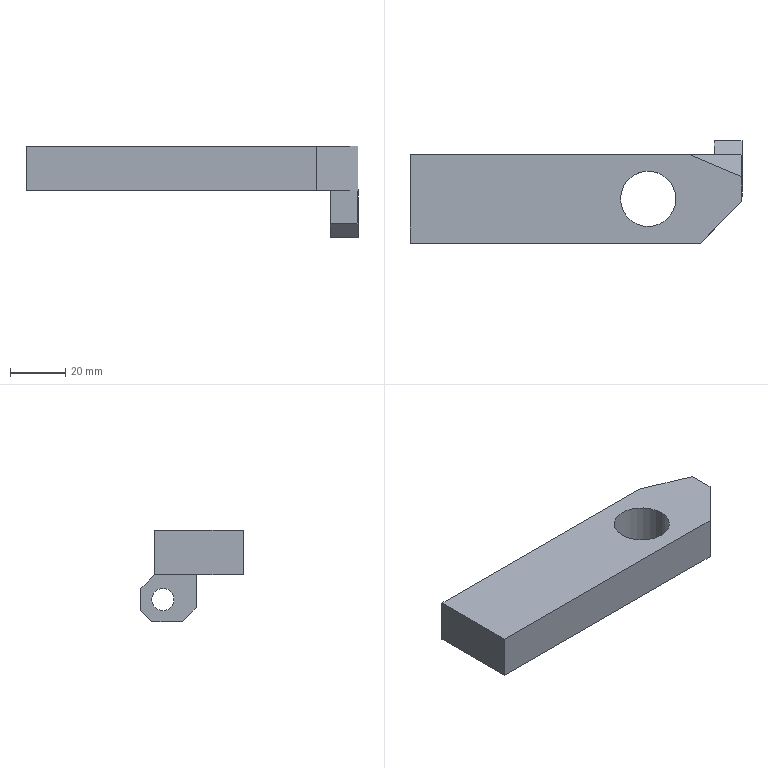Part | STEP file | [Anti-tilt]-Part-4 | 1 solid | 19 faces | box 120 x 37 x 33 mm | volume 56775 mm3 | plane 15 | cylinder 4 | commonest cylinder face diameters 8 x2 20 x2
STEP:
#1=CARTESIAN_POINT('',(63.91,-10.5,7.));
#2=VERTEX_POINT('',#1);
#3=CARTESIAN_POINT('',(63.91,-10.5,15.));
#4=VERTEX_POINT('',#3);
#5=CARTESIAN_POINT('',(63.91,-10.5,11.));
#6=DIRECTION('',(-1.,0.,0.));
#7=DIRECTION('',(0.,-1.,0.));
#8=AXIS2_PLACEMENT_3D('',#5,#6,#7);
#9=CIRCLE('',#8,4.);
#10=EDGE_CURVE('',#2,#4,#9,.T.);
#11=ORIENTED_EDGE('',*,*,#10,.F.);
#12=CARTESIAN_POINT('',(53.91,-10.5,7.));
#13=VERTEX_POINT('',#12);
#14=CARTESIAN_POINT('',(44.003,-10.5,7.));
#15=DIRECTION('',(-1.,0.,0.));
#16=VECTOR('',#15,1000.);
#17=LINE('',#14,#16);
#18=EDGE_CURVE('',#2,#13,#17,.T.);
#19=ORIENTED_EDGE('',*,*,#18,.T.);
#20=CARTESIAN_POINT('',(53.91,-10.5,15.));
#21=VERTEX_POINT('',#20);
#22=CARTESIAN_POINT('',(53.91,-10.5,11.));
#23=DIRECTION('',(1.,0.,0.));
#24=DIRECTION('',(0.,1.,0.));
#25=AXIS2_PLACEMENT_3D('',#22,#23,#24);
#26=CIRCLE('',#25,4.);
#27=EDGE_CURVE('',#21,#13,#26,.T.);
#28=ORIENTED_EDGE('',*,*,#27,.F.);
#29=CARTESIAN_POINT('',(44.003,-10.5,15.));
#30=DIRECTION('',(-1.,0.,0.));
#31=VECTOR('',#30,1000.);
#32=LINE('',#29,#31);
#33=EDGE_CURVE('',#4,#21,#32,.T.);
#34=ORIENTED_EDGE('',*,*,#33,.F.);
#35=EDGE_LOOP('',(#11,#19,#28,#34));
#36=FACE_OUTER_BOUND('',#35,.T.);
#37=CARTESIAN_POINT('',(44.003,-10.5,11.));
#38=DIRECTION('',(-1.,0.,0.));
#39=DIRECTION('',(0.,0.,1.));
#40=AXIS2_PLACEMENT_3D('',#37,#38,#39);
#41=CYLINDRICAL_SURFACE('',#40,4.);
#42=ADVANCED_FACE('',(#36),#41,.F.);
#43=CARTESIAN_POINT('',(40.003,-23.5,20.));
#44=VERTEX_POINT('',#43);
#45=CARTESIAN_POINT('',(20.003,-23.5,20.));
#46=VERTEX_POINT('',#45);
#47=CARTESIAN_POINT('',(30.003,-23.5,20.));
#48=DIRECTION('',(0.,0.,1.));
#49=DIRECTION('',(-1.,0.,0.));
#50=AXIS2_PLACEMENT_3D('',#47,#48,#49);
#51=CIRCLE('',#50,10.);
#52=EDGE_CURVE('',#44,#46,#51,.T.);
#53=ORIENTED_EDGE('',*,*,#52,.F.);
#54=CARTESIAN_POINT('',(40.003,-23.5,36.));
#55=VERTEX_POINT('',#54);
#56=CARTESIAN_POINT('',(40.003,-23.5,20.));
#57=DIRECTION('',(0.,0.,1.));
#58=VECTOR('',#57,1000.);
#59=LINE('',#56,#58);
#60=EDGE_CURVE('',#44,#55,#59,.T.);
#61=ORIENTED_EDGE('',*,*,#60,.T.);
#62=CARTESIAN_POINT('',(20.003,-23.5,36.));
#63=VERTEX_POINT('',#62);
#64=CARTESIAN_POINT('',(30.003,-23.5,36.));
#65=DIRECTION('',(0.,0.,1.));
#66=DIRECTION('',(-1.,0.,0.));
#67=AXIS2_PLACEMENT_3D('',#64,#65,#66);
#68=CIRCLE('',#67,10.);
#69=EDGE_CURVE('',#55,#63,#68,.T.);
#70=ORIENTED_EDGE('',*,*,#69,.T.);
#71=CARTESIAN_POINT('',(20.003,-23.5,20.));
#72=DIRECTION('',(0.,0.,1.));
#73=VECTOR('',#72,1000.);
#74=LINE('',#71,#73);
#75=EDGE_CURVE('',#46,#63,#74,.T.);
#76=ORIENTED_EDGE('',*,*,#75,.F.);
#77=EDGE_LOOP('',(#53,#61,#70,#76));
#78=FACE_OUTER_BOUND('',#77,.T.);
#79=CARTESIAN_POINT('',(30.003,-23.5,20.));
#80=DIRECTION('',(0.,0.,1.));
#81=DIRECTION('',(-1.,0.,0.));
#82=AXIS2_PLACEMENT_3D('',#79,#80,#81);
#83=CYLINDRICAL_SURFACE('',#82,10.);
#84=ADVANCED_FACE('',(#78),#83,.F.);
#85=CARTESIAN_POINT('',(30.003,-23.5,20.));
#86=DIRECTION('',(0.,0.,1.));
#87=DIRECTION('',(-1.,0.,0.));
#88=AXIS2_PLACEMENT_3D('',#85,#86,#87);
#89=CIRCLE('',#88,10.);
#90=EDGE_CURVE('',#46,#44,#89,.T.);
#91=ORIENTED_EDGE('',*,*,#90,.T.);
#92=ORIENTED_EDGE('',*,*,#52,.T.);
#93=EDGE_LOOP('',(#91,#92));
#94=FACE_BOUND('',#93,.T.);
#95=CARTESIAN_POINT('',(63.91,-22.5,20.));
#96=VERTEX_POINT('',#95);
#97=CARTESIAN_POINT('',(63.91,-24.5,20.));
#98=VERTEX_POINT('',#97);
#99=CARTESIAN_POINT('',(63.91,-23.5,20.));
#100=DIRECTION('',(0.,-1.,0.));
#101=VECTOR('',#100,1000.);
#102=LINE('',#99,#101);
#103=EDGE_CURVE('',#96,#98,#102,.T.);
#104=ORIENTED_EDGE('',*,*,#103,.T.);
#105=CARTESIAN_POINT('',(48.91,-39.5,20.));
#106=VERTEX_POINT('',#105);
#107=CARTESIAN_POINT('',(4.41,-84.,20.));
#108=DIRECTION('',(-0.7071,-0.7071,0.));
#109=VECTOR('',#108,1000.);
#110=LINE('',#107,#109);
#111=EDGE_CURVE('',#98,#106,#110,.T.);
#112=ORIENTED_EDGE('',*,*,#111,.T.);
#113=CARTESIAN_POINT('',(-56.09,-39.5,20.));
#114=VERTEX_POINT('',#113);
#115=CARTESIAN_POINT('',(-56.09,-39.5,20.));
#116=DIRECTION('',(1.,0.,0.));
#117=VECTOR('',#116,1000.);
#118=LINE('',#115,#117);
#119=EDGE_CURVE('',#114,#106,#118,.T.);
#120=ORIENTED_EDGE('',*,*,#119,.F.);
#121=CARTESIAN_POINT('',(-56.09,-7.5,20.));
#122=VERTEX_POINT('',#121);
#123=CARTESIAN_POINT('',(-56.09,-23.5,20.));
#124=DIRECTION('',(0.,1.,0.));
#125=VECTOR('',#124,1000.);
#126=LINE('',#123,#125);
#127=EDGE_CURVE('',#114,#122,#126,.T.);
#128=ORIENTED_EDGE('',*,*,#127,.T.);
#129=CARTESIAN_POINT('',(53.91,-7.5,20.));
#130=VERTEX_POINT('',#129);
#131=CARTESIAN_POINT('',(-56.09,-7.5,20.));
#132=DIRECTION('',(1.,0.,0.));
#133=VECTOR('',#132,1000.);
#134=LINE('',#131,#133);
#135=EDGE_CURVE('',#122,#130,#134,.T.);
#136=ORIENTED_EDGE('',*,*,#135,.T.);
#137=CARTESIAN_POINT('',(53.91,-22.5,20.));
#138=VERTEX_POINT('',#137);
#139=CARTESIAN_POINT('',(53.91,-12.5,20.));
#140=DIRECTION('',(0.,-1.,0.));
#141=VECTOR('',#140,1000.);
#142=LINE('',#139,#141);
#143=EDGE_CURVE('',#130,#138,#142,.T.);
#144=ORIENTED_EDGE('',*,*,#143,.T.);
#145=CARTESIAN_POINT('',(53.91,-22.5,20.));
#146=DIRECTION('',(1.,0.,0.));
#147=VECTOR('',#146,1000.);
#148=LINE('',#145,#147);
#149=EDGE_CURVE('',#138,#96,#148,.T.);
#150=ORIENTED_EDGE('',*,*,#149,.T.);
#151=EDGE_LOOP('',(#104,#112,#120,#128,#136,#144,#150));
#152=FACE_OUTER_BOUND('',#151,.T.);
#153=CARTESIAN_POINT('',(-56.09,-23.5,20.));
#154=DIRECTION('',(0.,0.,-1.));
#155=DIRECTION('',(1.,0.,0.));
#156=AXIS2_PLACEMENT_3D('',#153,#154,#155);
#157=PLANE('',#156);
#158=ADVANCED_FACE('',(#94,#152),#157,.T.);
#159=CARTESIAN_POINT('',(63.91,-24.5,36.));
#160=VERTEX_POINT('',#159);
#161=CARTESIAN_POINT('',(63.91,-15.5,36.));
#162=VERTEX_POINT('',#161);
#163=CARTESIAN_POINT('',(63.91,-23.5,36.));
#164=DIRECTION('',(0.,1.,0.));
#165=VECTOR('',#164,1000.);
#166=LINE('',#163,#165);
#167=EDGE_CURVE('',#160,#162,#166,.T.);
#168=ORIENTED_EDGE('',*,*,#167,.F.);
#169=CARTESIAN_POINT('',(63.91,-24.5,28.));
#170=DIRECTION('',(0.,0.,-1.));
#171=VECTOR('',#170,1000.);
#172=LINE('',#169,#171);
#173=EDGE_CURVE('',#160,#98,#172,.T.);
#174=ORIENTED_EDGE('',*,*,#173,.T.);
#175=ORIENTED_EDGE('',*,*,#103,.F.);
#176=CARTESIAN_POINT('',(63.91,-22.5,8.));
#177=VERTEX_POINT('',#176);
#178=CARTESIAN_POINT('',(63.91,-22.5,11.5));
#179=DIRECTION('',(0.,0.,1.));
#180=VECTOR('',#179,1000.);
#181=LINE('',#178,#180);
#182=EDGE_CURVE('',#177,#96,#181,.T.);
#183=ORIENTED_EDGE('',*,*,#182,.F.);
#184=CARTESIAN_POINT('',(63.91,-17.5,3.));
#185=VERTEX_POINT('',#184);
#186=CARTESIAN_POINT('',(63.91,-33.,18.5));
#187=DIRECTION('',(0.,0.7071,-0.7071));
#188=VECTOR('',#187,1000.);
#189=LINE('',#186,#188);
#190=EDGE_CURVE('',#177,#185,#189,.T.);
#191=ORIENTED_EDGE('',*,*,#190,.T.);
#192=CARTESIAN_POINT('',(63.91,-6.5,3.));
#193=VERTEX_POINT('',#192);
#194=CARTESIAN_POINT('',(63.91,-12.5,3.));
#195=DIRECTION('',(0.,-1.,0.));
#196=VECTOR('',#195,1000.);
#197=LINE('',#194,#196);
#198=EDGE_CURVE('',#193,#185,#197,.T.);
#199=ORIENTED_EDGE('',*,*,#198,.F.);
#200=CARTESIAN_POINT('',(63.91,-2.5,7.));
#201=VERTEX_POINT('',#200);
#202=CARTESIAN_POINT('',(63.91,-5.25,4.25));
#203=DIRECTION('',(0.,0.7071,0.7071));
#204=VECTOR('',#203,1000.);
#205=LINE('',#202,#204);
#206=EDGE_CURVE('',#193,#201,#205,.T.);
#207=ORIENTED_EDGE('',*,*,#206,.T.);
#208=CARTESIAN_POINT('',(63.91,-2.5,15.));
#209=VERTEX_POINT('',#208);
#210=CARTESIAN_POINT('',(63.91,-2.5,11.5));
#211=DIRECTION('',(0.,0.,-1.));
#212=VECTOR('',#211,1000.);
#213=LINE('',#210,#212);
#214=EDGE_CURVE('',#209,#201,#213,.T.);
#215=ORIENTED_EDGE('',*,*,#214,.F.);
#216=CARTESIAN_POINT('',(63.91,-7.5,20.));
#217=VERTEX_POINT('',#216);
#218=CARTESIAN_POINT('',(63.91,-5.75,18.25));
#219=DIRECTION('',(0.,-0.7071,0.7071));
#220=VECTOR('',#219,1000.);
#221=LINE('',#218,#220);
#222=EDGE_CURVE('',#209,#217,#221,.T.);
#223=ORIENTED_EDGE('',*,*,#222,.T.);
#224=CARTESIAN_POINT('',(63.91,-13.9,32.8));
#225=DIRECTION('',(0.,0.4472,-0.8944));
#226=VECTOR('',#225,1000.);
#227=LINE('',#224,#226);
#228=EDGE_CURVE('',#162,#217,#227,.T.);
#229=ORIENTED_EDGE('',*,*,#228,.F.);
#230=EDGE_LOOP('',(#168,#174,#175,#183,#191,#199,#207,#215,#223,#229));
#231=FACE_OUTER_BOUND('',#230,.T.);
#232=CARTESIAN_POINT('',(63.91,-10.5,11.));
#233=DIRECTION('',(-1.,0.,0.));
#234=DIRECTION('',(0.,-1.,0.));
#235=AXIS2_PLACEMENT_3D('',#232,#233,#234);
#236=CIRCLE('',#235,4.);
#237=EDGE_CURVE('',#4,#2,#236,.T.);
#238=ORIENTED_EDGE('',*,*,#237,.T.);
#239=ORIENTED_EDGE('',*,*,#10,.T.);
#240=EDGE_LOOP('',(#238,#239));
#241=FACE_BOUND('',#240,.T.);
#242=CARTESIAN_POINT('',(63.91,-23.5,28.));
#243=DIRECTION('',(1.,0.,0.));
#244=DIRECTION('',(0.,-1.,0.));
#245=AXIS2_PLACEMENT_3D('',#242,#243,#244);
#246=PLANE('',#245);
#247=ADVANCED_FACE('',(#231,#241),#246,.T.);
#248=CARTESIAN_POINT('',(-56.09,-39.5,36.));
#249=VERTEX_POINT('',#248);
#250=CARTESIAN_POINT('',(48.91,-39.5,36.));
#251=VERTEX_POINT('',#250);
#252=CARTESIAN_POINT('',(-56.09,-39.5,36.));
#253=DIRECTION('',(1.,0.,0.));
#254=VECTOR('',#253,1000.);
#255=LINE('',#252,#254);
#256=EDGE_CURVE('',#249,#251,#255,.T.);
#257=ORIENTED_EDGE('',*,*,#256,.T.);
#258=CARTESIAN_POINT('',(4.41,-84.,36.));
#259=DIRECTION('',(0.7071,0.7071,0.));
#260=VECTOR('',#259,1000.);
#261=LINE('',#258,#260);
#262=EDGE_CURVE('',#251,#160,#261,.T.);
#263=ORIENTED_EDGE('',*,*,#262,.T.);
#264=ORIENTED_EDGE('',*,*,#167,.T.);
#265=CARTESIAN_POINT('',(44.91,-7.5,36.));
#266=VERTEX_POINT('',#265);
#267=CARTESIAN_POINT('',(50.086,-9.68,36.));
#268=DIRECTION('',(0.9216,-0.3881,0.));
#269=VECTOR('',#268,1000.);
#270=LINE('',#267,#269);
#271=EDGE_CURVE('',#266,#162,#270,.T.);
#272=ORIENTED_EDGE('',*,*,#271,.F.);
#273=CARTESIAN_POINT('',(-56.09,-7.5,36.));
#274=VERTEX_POINT('',#273);
#275=CARTESIAN_POINT('',(-56.09,-7.5,36.));
#276=DIRECTION('',(1.,0.,0.));
#277=VECTOR('',#276,1000.);
#278=LINE('',#275,#277);
#279=EDGE_CURVE('',#274,#266,#278,.T.);
#280=ORIENTED_EDGE('',*,*,#279,.F.);
#281=CARTESIAN_POINT('',(-56.09,-23.5,36.));
#282=DIRECTION('',(0.,-1.,0.));
#283=VECTOR('',#282,1000.);
#284=LINE('',#281,#283);
#285=EDGE_CURVE('',#274,#249,#284,.T.);
#286=ORIENTED_EDGE('',*,*,#285,.T.);
#287=EDGE_LOOP('',(#257,#263,#264,#272,#280,#286));
#288=FACE_OUTER_BOUND('',#287,.T.);
#289=CARTESIAN_POINT('',(30.003,-23.5,36.));
#290=DIRECTION('',(0.,0.,1.));
#291=DIRECTION('',(-1.,0.,0.));
#292=AXIS2_PLACEMENT_3D('',#289,#290,#291);
#293=CIRCLE('',#292,10.);
#294=EDGE_CURVE('',#63,#55,#293,.T.);
#295=ORIENTED_EDGE('',*,*,#294,.F.);
#296=ORIENTED_EDGE('',*,*,#69,.F.);
#297=EDGE_LOOP('',(#295,#296));
#298=FACE_BOUND('',#297,.T.);
#299=CARTESIAN_POINT('',(-56.09,-23.5,36.));
#300=DIRECTION('',(0.,0.,1.));
#301=DIRECTION('',(-1.,0.,0.));
#302=AXIS2_PLACEMENT_3D('',#299,#300,#301);
#303=PLANE('',#302);
#304=ADVANCED_FACE('',(#288,#298),#303,.T.);
#305=CARTESIAN_POINT('',(-10.242,-7.5,82.444));
#306=DIRECTION('',(-0.7649,0.,0.6441));
#307=VECTOR('',#306,1000.);
#308=LINE('',#305,#307);
#309=EDGE_CURVE('',#217,#266,#308,.T.);
#310=ORIENTED_EDGE('',*,*,#309,.F.);
#311=CARTESIAN_POINT('',(53.91,-7.5,20.));
#312=DIRECTION('',(-1.,0.,0.));
#313=VECTOR('',#312,1000.);
#314=LINE('',#311,#313);
#315=EDGE_CURVE('',#217,#130,#314,.T.);
#316=ORIENTED_EDGE('',*,*,#315,.T.);
#317=ORIENTED_EDGE('',*,*,#135,.F.);
#318=CARTESIAN_POINT('',(-56.09,-7.5,28.));
#319=DIRECTION('',(0.,0.,1.));
#320=VECTOR('',#319,1000.);
#321=LINE('',#318,#320);
#322=EDGE_CURVE('',#122,#274,#321,.T.);
#323=ORIENTED_EDGE('',*,*,#322,.T.);
#324=ORIENTED_EDGE('',*,*,#279,.T.);
#325=EDGE_LOOP('',(#310,#316,#317,#323,#324));
#326=FACE_OUTER_BOUND('',#325,.T.);
#327=CARTESIAN_POINT('',(-56.09,-7.5,28.));
#328=DIRECTION('',(0.,1.,0.));
#329=DIRECTION('',(1.,0.,0.));
#330=AXIS2_PLACEMENT_3D('',#327,#328,#329);
#331=PLANE('',#330);
#332=ADVANCED_FACE('',(#326),#331,.T.);
#333=CARTESIAN_POINT('',(-56.09,-39.5,28.));
#334=DIRECTION('',(0.,0.,-1.));
#335=VECTOR('',#334,1000.);
#336=LINE('',#333,#335);
#337=EDGE_CURVE('',#249,#114,#336,.T.);
#338=ORIENTED_EDGE('',*,*,#337,.F.);
#339=ORIENTED_EDGE('',*,*,#285,.F.);
#340=ORIENTED_EDGE('',*,*,#322,.F.);
#341=ORIENTED_EDGE('',*,*,#127,.F.);
#342=EDGE_LOOP('',(#338,#339,#340,#341));
#343=FACE_OUTER_BOUND('',#342,.T.);
#344=CARTESIAN_POINT('',(-56.09,-23.5,28.));
#345=DIRECTION('',(-1.,0.,0.));
#346=DIRECTION('',(0.,1.,0.));
#347=AXIS2_PLACEMENT_3D('',#344,#345,#346);
#348=PLANE('',#347);
#349=ADVANCED_FACE('',(#343),#348,.T.);
#350=ORIENTED_EDGE('',*,*,#119,.T.);
#351=CARTESIAN_POINT('',(48.91,-39.5,28.));
#352=DIRECTION('',(0.,0.,1.));
#353=VECTOR('',#352,1000.);
#354=LINE('',#351,#353);
#355=EDGE_CURVE('',#106,#251,#354,.T.);
#356=ORIENTED_EDGE('',*,*,#355,.T.);
#357=ORIENTED_EDGE('',*,*,#256,.F.);
#358=ORIENTED_EDGE('',*,*,#337,.T.);
#359=EDGE_LOOP('',(#350,#356,#357,#358));
#360=FACE_OUTER_BOUND('',#359,.T.);
#361=CARTESIAN_POINT('',(-56.09,-39.5,28.));
#362=DIRECTION('',(0.,-1.,0.));
#363=DIRECTION('',(-1.,0.,0.));
#364=AXIS2_PLACEMENT_3D('',#361,#362,#363);
#365=PLANE('',#364);
#366=ADVANCED_FACE('',(#360),#365,.T.);
#367=ORIENTED_EDGE('',*,*,#60,.F.);
#368=ORIENTED_EDGE('',*,*,#90,.F.);
#369=ORIENTED_EDGE('',*,*,#75,.T.);
#370=ORIENTED_EDGE('',*,*,#294,.T.);
#371=EDGE_LOOP('',(#367,#368,#369,#370));
#372=FACE_OUTER_BOUND('',#371,.T.);
#373=CARTESIAN_POINT('',(30.003,-23.5,20.));
#374=DIRECTION('',(0.,0.,1.));
#375=DIRECTION('',(-1.,0.,0.));
#376=AXIS2_PLACEMENT_3D('',#373,#374,#375);
#377=CYLINDRICAL_SURFACE('',#376,10.);
#378=ADVANCED_FACE('',(#372),#377,.F.);
#379=ORIENTED_EDGE('',*,*,#228,.T.);
#380=ORIENTED_EDGE('',*,*,#309,.T.);
#381=ORIENTED_EDGE('',*,*,#271,.T.);
#382=EDGE_LOOP('',(#379,#380,#381));
#383=FACE_OUTER_BOUND('',#382,.T.);
#384=CARTESIAN_POINT('',(51.71,-5.822,26.918));
#385=DIRECTION('',(-0.3524,-0.837,-0.4185));
#386=DIRECTION('',(-0.9216,0.3881,0.));
#387=AXIS2_PLACEMENT_3D('',#384,#385,#386);
#388=PLANE('',#387);
#389=ADVANCED_FACE('',(#383),#388,.F.);
#390=ORIENTED_EDGE('',*,*,#214,.T.);
#391=CARTESIAN_POINT('',(53.91,-2.5,7.));
#392=VERTEX_POINT('',#391);
#393=CARTESIAN_POINT('',(53.91,-2.5,7.));
#394=DIRECTION('',(-1.,0.,0.));
#395=VECTOR('',#394,1000.);
#396=LINE('',#393,#395);
#397=EDGE_CURVE('',#201,#392,#396,.T.);
#398=ORIENTED_EDGE('',*,*,#397,.T.);
#399=CARTESIAN_POINT('',(53.91,-2.5,15.));
#400=VERTEX_POINT('',#399);
#401=CARTESIAN_POINT('',(53.91,-2.5,11.5));
#402=DIRECTION('',(0.,0.,1.));
#403=VECTOR('',#402,1000.);
#404=LINE('',#401,#403);
#405=EDGE_CURVE('',#392,#400,#404,.T.);
#406=ORIENTED_EDGE('',*,*,#405,.T.);
#407=CARTESIAN_POINT('',(53.91,-2.5,15.));
#408=DIRECTION('',(1.,0.,0.));
#409=VECTOR('',#408,1000.);
#410=LINE('',#407,#409);
#411=EDGE_CURVE('',#400,#209,#410,.T.);
#412=ORIENTED_EDGE('',*,*,#411,.T.);
#413=EDGE_LOOP('',(#390,#398,#406,#412));
#414=FACE_OUTER_BOUND('',#413,.T.);
#415=CARTESIAN_POINT('',(53.91,-2.5,11.5));
#416=DIRECTION('',(0.,1.,0.));
#417=DIRECTION('',(1.,0.,0.));
#418=AXIS2_PLACEMENT_3D('',#415,#416,#417);
#419=PLANE('',#418);
#420=ADVANCED_FACE('',(#414),#419,.T.);
#421=ORIENTED_EDGE('',*,*,#198,.T.);
#422=CARTESIAN_POINT('',(53.91,-17.5,3.));
#423=VERTEX_POINT('',#422);
#424=CARTESIAN_POINT('',(53.91,-17.5,3.));
#425=DIRECTION('',(-1.,0.,0.));
#426=VECTOR('',#425,1000.);
#427=LINE('',#424,#426);
#428=EDGE_CURVE('',#185,#423,#427,.T.);
#429=ORIENTED_EDGE('',*,*,#428,.T.);
#430=CARTESIAN_POINT('',(53.91,-6.5,3.));
#431=VERTEX_POINT('',#430);
#432=CARTESIAN_POINT('',(53.91,-12.5,3.));
#433=DIRECTION('',(0.,1.,0.));
#434=VECTOR('',#433,1000.);
#435=LINE('',#432,#434);
#436=EDGE_CURVE('',#423,#431,#435,.T.);
#437=ORIENTED_EDGE('',*,*,#436,.T.);
#438=CARTESIAN_POINT('',(53.91,-6.5,3.));
#439=DIRECTION('',(1.,0.,0.));
#440=VECTOR('',#439,1000.);
#441=LINE('',#438,#440);
#442=EDGE_CURVE('',#431,#193,#441,.T.);
#443=ORIENTED_EDGE('',*,*,#442,.T.);
#444=EDGE_LOOP('',(#421,#429,#437,#443));
#445=FACE_OUTER_BOUND('',#444,.T.);
#446=CARTESIAN_POINT('',(53.91,-12.5,3.));
#447=DIRECTION('',(0.,0.,-1.));
#448=DIRECTION('',(1.,0.,0.));
#449=AXIS2_PLACEMENT_3D('',#446,#447,#448);
#450=PLANE('',#449);
#451=ADVANCED_FACE('',(#445),#450,.T.);
#452=ORIENTED_EDGE('',*,*,#27,.T.);
#453=CARTESIAN_POINT('',(53.91,-10.5,11.));
#454=DIRECTION('',(1.,0.,0.));
#455=DIRECTION('',(0.,1.,0.));
#456=AXIS2_PLACEMENT_3D('',#453,#454,#455);
#457=CIRCLE('',#456,4.);
#458=EDGE_CURVE('',#13,#21,#457,.T.);
#459=ORIENTED_EDGE('',*,*,#458,.T.);
#460=EDGE_LOOP('',(#452,#459));
#461=FACE_BOUND('',#460,.T.);
#462=ORIENTED_EDGE('',*,*,#436,.F.);
#463=CARTESIAN_POINT('',(53.91,-22.5,8.));
#464=VERTEX_POINT('',#463);
#465=CARTESIAN_POINT('',(53.91,-19.25,4.75));
#466=DIRECTION('',(0.,-0.7071,0.7071));
#467=VECTOR('',#466,1000.);
#468=LINE('',#465,#467);
#469=EDGE_CURVE('',#423,#464,#468,.T.);
#470=ORIENTED_EDGE('',*,*,#469,.T.);
#471=CARTESIAN_POINT('',(53.91,-22.5,11.5));
#472=DIRECTION('',(0.,0.,-1.));
#473=VECTOR('',#472,1000.);
#474=LINE('',#471,#473);
#475=EDGE_CURVE('',#138,#464,#474,.T.);
#476=ORIENTED_EDGE('',*,*,#475,.F.);
#477=ORIENTED_EDGE('',*,*,#143,.F.);
#478=CARTESIAN_POINT('',(53.91,-5.75,18.25));
#479=DIRECTION('',(0.,0.7071,-0.7071));
#480=VECTOR('',#479,1000.);
#481=LINE('',#478,#480);
#482=EDGE_CURVE('',#130,#400,#481,.T.);
#483=ORIENTED_EDGE('',*,*,#482,.T.);
#484=ORIENTED_EDGE('',*,*,#405,.F.);
#485=CARTESIAN_POINT('',(53.91,-5.25,4.25));
#486=DIRECTION('',(0.,-0.7071,-0.7071));
#487=VECTOR('',#486,1000.);
#488=LINE('',#485,#487);
#489=EDGE_CURVE('',#392,#431,#488,.T.);
#490=ORIENTED_EDGE('',*,*,#489,.T.);
#491=EDGE_LOOP('',(#462,#470,#476,#477,#483,#484,#490));
#492=FACE_OUTER_BOUND('',#491,.T.);
#493=CARTESIAN_POINT('',(53.91,-12.5,11.5));
#494=DIRECTION('',(-1.,0.,0.));
#495=DIRECTION('',(0.,1.,0.));
#496=AXIS2_PLACEMENT_3D('',#493,#494,#495);
#497=PLANE('',#496);
#498=ADVANCED_FACE('',(#461,#492),#497,.T.);
#499=ORIENTED_EDGE('',*,*,#475,.T.);
#500=CARTESIAN_POINT('',(53.91,-22.5,8.));
#501=DIRECTION('',(1.,0.,0.));
#502=VECTOR('',#501,1000.);
#503=LINE('',#500,#502);
#504=EDGE_CURVE('',#464,#177,#503,.T.);
#505=ORIENTED_EDGE('',*,*,#504,.T.);
#506=ORIENTED_EDGE('',*,*,#182,.T.);
#507=ORIENTED_EDGE('',*,*,#149,.F.);
#508=EDGE_LOOP('',(#499,#505,#506,#507));
#509=FACE_OUTER_BOUND('',#508,.T.);
#510=CARTESIAN_POINT('',(53.91,-22.5,11.5));
#511=DIRECTION('',(0.,-1.,0.));
#512=DIRECTION('',(-1.,0.,0.));
#513=AXIS2_PLACEMENT_3D('',#510,#511,#512);
#514=PLANE('',#513);
#515=ADVANCED_FACE('',(#509),#514,.T.);
#516=ORIENTED_EDGE('',*,*,#482,.F.);
#517=ORIENTED_EDGE('',*,*,#315,.F.);
#518=ORIENTED_EDGE('',*,*,#222,.F.);
#519=ORIENTED_EDGE('',*,*,#411,.F.);
#520=EDGE_LOOP('',(#516,#517,#518,#519));
#521=FACE_OUTER_BOUND('',#520,.T.);
#522=CARTESIAN_POINT('',(53.91,-2.5,15.));
#523=DIRECTION('',(0.,-0.7071,-0.7071));
#524=DIRECTION('',(1.,0.,0.));
#525=AXIS2_PLACEMENT_3D('',#522,#523,#524);
#526=PLANE('',#525);
#527=ADVANCED_FACE('',(#521),#526,.F.);
#528=ORIENTED_EDGE('',*,*,#489,.F.);
#529=ORIENTED_EDGE('',*,*,#397,.F.);
#530=ORIENTED_EDGE('',*,*,#206,.F.);
#531=ORIENTED_EDGE('',*,*,#442,.F.);
#532=EDGE_LOOP('',(#528,#529,#530,#531));
#533=FACE_OUTER_BOUND('',#532,.T.);
#534=CARTESIAN_POINT('',(53.91,-6.5,3.));
#535=DIRECTION('',(0.,-0.7071,0.7071));
#536=DIRECTION('',(1.,0.,0.));
#537=AXIS2_PLACEMENT_3D('',#534,#535,#536);
#538=PLANE('',#537);
#539=ADVANCED_FACE('',(#533),#538,.F.);
#540=ORIENTED_EDGE('',*,*,#18,.F.);
#541=ORIENTED_EDGE('',*,*,#237,.F.);
#542=ORIENTED_EDGE('',*,*,#33,.T.);
#543=ORIENTED_EDGE('',*,*,#458,.F.);
#544=EDGE_LOOP('',(#540,#541,#542,#543));
#545=FACE_OUTER_BOUND('',#544,.T.);
#546=CARTESIAN_POINT('',(44.003,-10.5,11.));
#547=DIRECTION('',(-1.,0.,0.));
#548=DIRECTION('',(0.,0.,1.));
#549=AXIS2_PLACEMENT_3D('',#546,#547,#548);
#550=CYLINDRICAL_SURFACE('',#549,4.);
#551=ADVANCED_FACE('',(#545),#550,.F.);
#552=ORIENTED_EDGE('',*,*,#469,.F.);
#553=ORIENTED_EDGE('',*,*,#428,.F.);
#554=ORIENTED_EDGE('',*,*,#190,.F.);
#555=ORIENTED_EDGE('',*,*,#504,.F.);
#556=EDGE_LOOP('',(#552,#553,#554,#555));
#557=FACE_OUTER_BOUND('',#556,.T.);
#558=CARTESIAN_POINT('',(53.91,-22.5,8.));
#559=DIRECTION('',(0.,0.7071,0.7071));
#560=DIRECTION('',(1.,0.,0.));
#561=AXIS2_PLACEMENT_3D('',#558,#559,#560);
#562=PLANE('',#561);
#563=ADVANCED_FACE('',(#557),#562,.F.);
#564=ORIENTED_EDGE('',*,*,#111,.F.);
#565=ORIENTED_EDGE('',*,*,#173,.F.);
#566=ORIENTED_EDGE('',*,*,#262,.F.);
#567=ORIENTED_EDGE('',*,*,#355,.F.);
#568=EDGE_LOOP('',(#564,#565,#566,#567));
#569=FACE_OUTER_BOUND('',#568,.T.);
#570=CARTESIAN_POINT('',(48.91,-39.5,28.));
#571=DIRECTION('',(-0.7071,0.7071,0.));
#572=DIRECTION('',(0.,0.,1.));
#573=AXIS2_PLACEMENT_3D('',#570,#571,#572);
#574=PLANE('',#573);
#575=ADVANCED_FACE('',(#569),#574,.F.);
#576=CLOSED_SHELL('',(#42,#84,#158,#247,#304,#332,#349,#366,#378,#389,#420,#451,#498,#515,#527,#539,#551,#563,#575));
#577=MANIFOLD_SOLID_BREP('',#576);
#578=CARTESIAN_POINT('',(0.,0.,0.));
#579=DIRECTION('',(0.,0.,1.));
#580=DIRECTION('',(1.,0.,0.));
#581=AXIS2_PLACEMENT_3D('',#578,#579,#580);
#582=(LENGTH_UNIT()NAMED_UNIT(*)SI_UNIT(.MILLI.,.METRE.));
#583=UNCERTAINTY_MEASURE_WITH_UNIT(LENGTH_MEASURE(0.00001),#582,'','');
#584=(NAMED_UNIT(*)PLANE_ANGLE_UNIT()SI_UNIT($,.RADIAN.));
#585=(NAMED_UNIT(*)SI_UNIT($,.STERADIAN.)SOLID_ANGLE_UNIT());
#586=(GEOMETRIC_REPRESENTATION_CONTEXT(3)GLOBAL_UNCERTAINTY_ASSIGNED_CONTEXT((#583))GLOBAL_UNIT_ASSIGNED_CONTEXT((#582,#584,#585))REPRESENTATION_CONTEXT('',''));
#587=ADVANCED_BREP_SHAPE_REPRESENTATION('',(#577,#581),#586);